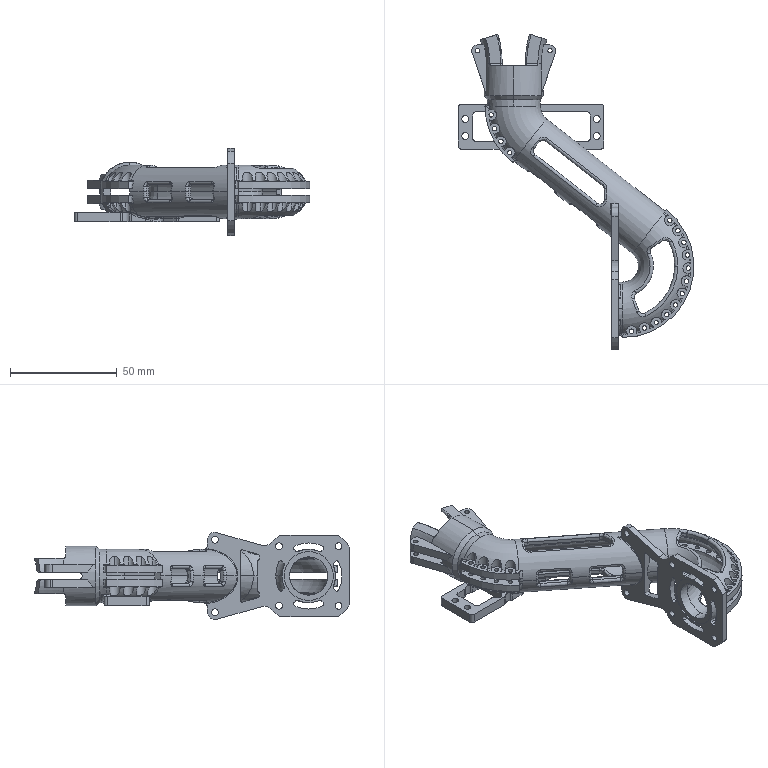Part | SolidWorks | 2 solids | 678 faces | box 110.5 x 147.904 x 41 mm | volume 42458 mm3 | cylinder 328 | spline 121 | plane 117 | torus 110 | cone 2 | commonest cylinder face diameters 2.1 x72 2 x67 5 x64 3.2 x20 3 x19 4 x18